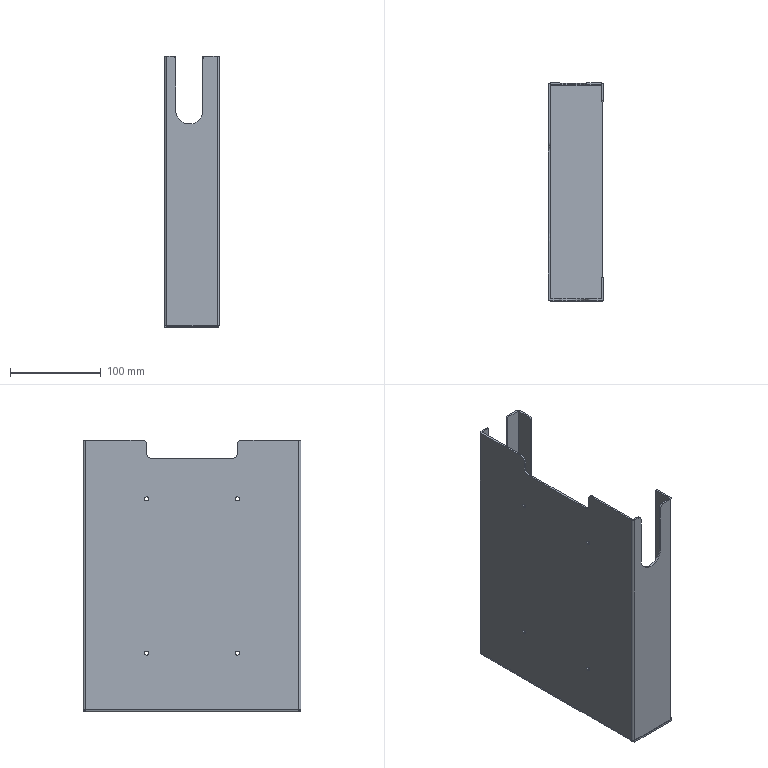Part | STEP file | DX-300 | 1 solid | 62 faces | box 61 x 240 x 300 mm | volume 251814 mm3 | plane 34 | cylinder 28 | commonest cylinder face diameters 4.5 x8 10 x6 1 x5 5 x5 4 x2 30 x2